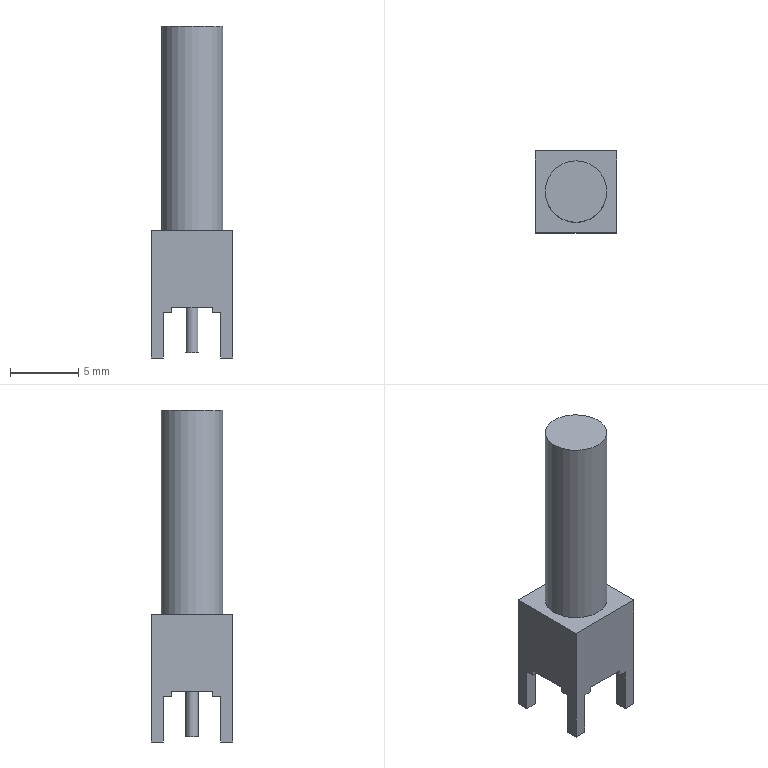Part | STEP file | MCX-KHD20 | 1 solid | 34 faces | box 6 x 6 x 24.3 mm | volume 456.556 mm3 | plane 32 | cylinder 2 | commonest cylinder face diameters 0.9 x1 4.5 x1